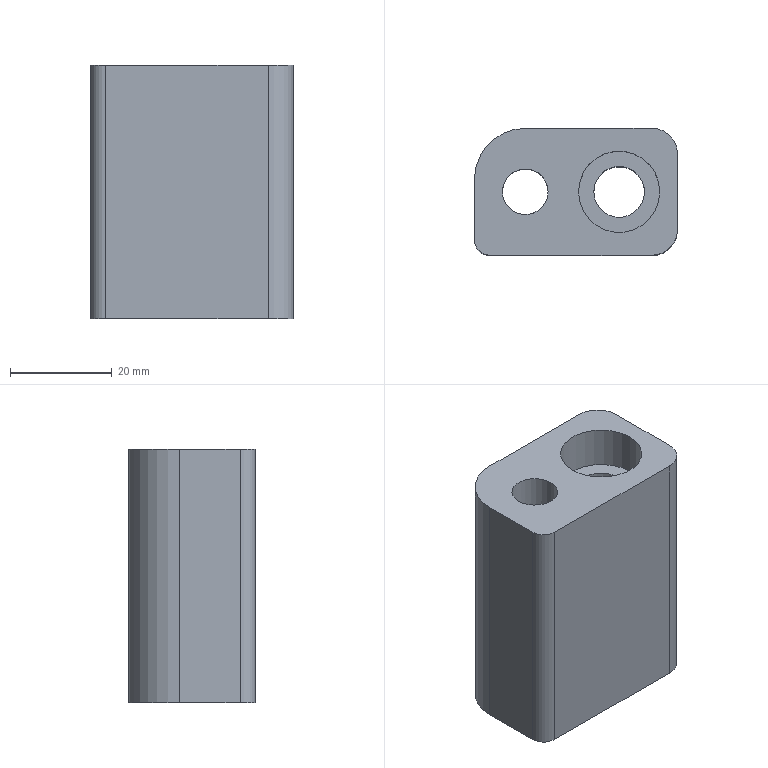Part | STEP file | PN_0016_id882_x_t | 1 solid | 16 faces | box 40 x 25 x 50 mm | volume 37460 mm3 | plane 8 | cylinder 8 | commonest cylinder face diameters 10 x3 6 x1 9 x1 14 x1 16 x1 20 x1
STEP:
#1=CARTESIAN_POINT('',(-201.,0.,95.));
#2=VERTEX_POINT('',#1);
#3=CARTESIAN_POINT('',(-209.,0.,95.));
#4=DIRECTION('',(0.,0.,-1.));
#5=DIRECTION('',(1.,0.,0.));
#6=AXIS2_PLACEMENT_3D('',#3,#4,#5);
#7=CIRCLE('',#6,8.);
#8=EDGE_CURVE('',#2,#2,#7,.T.);
#9=ORIENTED_EDGE('',*,*,#8,.T.);
#10=EDGE_LOOP('',(#9));
#11=FACE_BOUND('',#10,.T.);
#12=CARTESIAN_POINT('',(-223.,0.,95.));
#13=VERTEX_POINT('',#12);
#14=CARTESIAN_POINT('',(-227.5,0.,95.));
#15=DIRECTION('',(0.,0.,1.));
#16=DIRECTION('',(1.,0.,0.));
#17=AXIS2_PLACEMENT_3D('',#14,#15,#16);
#18=CIRCLE('',#17,4.5);
#19=EDGE_CURVE('',#13,#13,#18,.T.);
#20=ORIENTED_EDGE('',*,*,#19,.F.);
#21=EDGE_LOOP('',(#20));
#22=FACE_BOUND('',#21,.T.);
#23=CARTESIAN_POINT('',(-237.5,-9.5,95.));
#24=VERTEX_POINT('',#23);
#25=CARTESIAN_POINT('',(-237.5,2.5,95.));
#26=VERTEX_POINT('',#25);
#27=CARTESIAN_POINT('',(-237.5,0.,95.));
#28=DIRECTION('',(0.,1.,0.));
#29=VECTOR('',#28,1.);
#30=LINE('',#27,#29);
#31=EDGE_CURVE('',#24,#26,#30,.T.);
#32=ORIENTED_EDGE('',*,*,#31,.F.);
#33=CARTESIAN_POINT('',(-234.5,-12.5,95.));
#34=VERTEX_POINT('',#33);
#35=CARTESIAN_POINT('',(-234.5,-9.5,95.));
#36=DIRECTION('',(0.,0.,1.));
#37=DIRECTION('',(1.,0.,0.));
#38=AXIS2_PLACEMENT_3D('',#35,#36,#37);
#39=CIRCLE('',#38,3.);
#40=EDGE_CURVE('',#24,#34,#39,.T.);
#41=ORIENTED_EDGE('',*,*,#40,.T.);
#42=CARTESIAN_POINT('',(-202.5,-12.5,95.));
#43=VERTEX_POINT('',#42);
#44=CARTESIAN_POINT('',(-209.,-12.5,95.));
#45=DIRECTION('',(-1.,0.,0.));
#46=VECTOR('',#45,1.);
#47=LINE('',#44,#46);
#48=EDGE_CURVE('',#43,#34,#47,.T.);
#49=ORIENTED_EDGE('',*,*,#48,.F.);
#50=CARTESIAN_POINT('',(-197.5,-7.5,95.));
#51=VERTEX_POINT('',#50);
#52=CARTESIAN_POINT('',(-202.5,-7.5,95.));
#53=DIRECTION('',(0.,0.,1.));
#54=DIRECTION('',(1.,0.,0.));
#55=AXIS2_PLACEMENT_3D('',#52,#53,#54);
#56=CIRCLE('',#55,5.);
#57=EDGE_CURVE('',#43,#51,#56,.T.);
#58=ORIENTED_EDGE('',*,*,#57,.T.);
#59=CARTESIAN_POINT('',(-197.5,7.5,95.));
#60=VERTEX_POINT('',#59);
#61=CARTESIAN_POINT('',(-197.5,0.,95.));
#62=DIRECTION('',(0.,-1.,0.));
#63=VECTOR('',#62,1.);
#64=LINE('',#61,#63);
#65=EDGE_CURVE('',#60,#51,#64,.T.);
#66=ORIENTED_EDGE('',*,*,#65,.F.);
#67=CARTESIAN_POINT('',(-202.5,12.5,95.));
#68=VERTEX_POINT('',#67);
#69=CARTESIAN_POINT('',(-202.5,7.5,95.));
#70=DIRECTION('',(0.,0.,1.));
#71=DIRECTION('',(1.,0.,0.));
#72=AXIS2_PLACEMENT_3D('',#69,#70,#71);
#73=CIRCLE('',#72,5.);
#74=EDGE_CURVE('',#60,#68,#73,.T.);
#75=ORIENTED_EDGE('',*,*,#74,.T.);
#76=CARTESIAN_POINT('',(-227.5,12.5,95.));
#77=VERTEX_POINT('',#76);
#78=CARTESIAN_POINT('',(-209.,12.5,95.));
#79=DIRECTION('',(1.,0.,0.));
#80=VECTOR('',#79,1.);
#81=LINE('',#78,#80);
#82=EDGE_CURVE('',#77,#68,#81,.T.);
#83=ORIENTED_EDGE('',*,*,#82,.F.);
#84=CARTESIAN_POINT('',(-227.5,2.5,95.));
#85=DIRECTION('',(0.,0.,1.));
#86=DIRECTION('',(1.,0.,0.));
#87=AXIS2_PLACEMENT_3D('',#84,#85,#86);
#88=CIRCLE('',#87,10.);
#89=EDGE_CURVE('',#77,#26,#88,.T.);
#90=ORIENTED_EDGE('',*,*,#89,.T.);
#91=EDGE_LOOP('',(#32,#41,#49,#58,#66,#75,#83,#90));
#92=FACE_BOUND('',#91,.T.);
#93=CARTESIAN_POINT('',(-209.,0.,95.));
#94=DIRECTION('',(0.,0.,1.));
#95=DIRECTION('',(0.,-1.,0.));
#96=AXIS2_PLACEMENT_3D('',#93,#94,#95);
#97=PLANE('',#96);
#98=ADVANCED_FACE('',(#11,#22,#92),#97,.T.);
#99=CARTESIAN_POINT('',(-237.5,2.5,45.));
#100=VERTEX_POINT('',#99);
#101=CARTESIAN_POINT('',(-237.5,-9.5,45.));
#102=VERTEX_POINT('',#101);
#103=CARTESIAN_POINT('',(-237.5,0.,45.));
#104=DIRECTION('',(0.,-1.,0.));
#105=VECTOR('',#104,1.);
#106=LINE('',#103,#105);
#107=EDGE_CURVE('',#100,#102,#106,.T.);
#108=ORIENTED_EDGE('',*,*,#107,.T.);
#109=CARTESIAN_POINT('',(-237.5,-9.5,5.));
#110=DIRECTION('',(0.,0.,1.));
#111=VECTOR('',#110,1.);
#112=LINE('',#109,#111);
#113=EDGE_CURVE('',#102,#24,#112,.T.);
#114=ORIENTED_EDGE('',*,*,#113,.T.);
#115=ORIENTED_EDGE('',*,*,#31,.T.);
#116=CARTESIAN_POINT('',(-237.5,2.5,5.));
#117=DIRECTION('',(0.,0.,-1.));
#118=VECTOR('',#117,1.);
#119=LINE('',#116,#118);
#120=EDGE_CURVE('',#26,#100,#119,.T.);
#121=ORIENTED_EDGE('',*,*,#120,.T.);
#122=EDGE_LOOP('',(#108,#114,#115,#121));
#123=FACE_OUTER_BOUND('',#122,.T.);
#124=CARTESIAN_POINT('',(-237.5,0.,5.));
#125=DIRECTION('',(-1.,0.,0.));
#126=DIRECTION('',(0.,0.,-1.));
#127=AXIS2_PLACEMENT_3D('',#124,#125,#126);
#128=PLANE('',#127);
#129=ADVANCED_FACE('',(#123),#128,.T.);
#130=CARTESIAN_POINT('',(-202.5,12.5,45.));
#131=VERTEX_POINT('',#130);
#132=CARTESIAN_POINT('',(-227.5,12.5,45.));
#133=VERTEX_POINT('',#132);
#134=CARTESIAN_POINT('',(-209.,12.5,45.));
#135=DIRECTION('',(-1.,0.,0.));
#136=VECTOR('',#135,1.);
#137=LINE('',#134,#136);
#138=EDGE_CURVE('',#131,#133,#137,.T.);
#139=ORIENTED_EDGE('',*,*,#138,.T.);
#140=CARTESIAN_POINT('',(-227.5,12.5,5.));
#141=DIRECTION('',(0.,0.,1.));
#142=VECTOR('',#141,1.);
#143=LINE('',#140,#142);
#144=EDGE_CURVE('',#133,#77,#143,.T.);
#145=ORIENTED_EDGE('',*,*,#144,.T.);
#146=ORIENTED_EDGE('',*,*,#82,.T.);
#147=CARTESIAN_POINT('',(-202.5,12.5,5.));
#148=DIRECTION('',(0.,0.,-1.));
#149=VECTOR('',#148,1.);
#150=LINE('',#147,#149);
#151=EDGE_CURVE('',#68,#131,#150,.T.);
#152=ORIENTED_EDGE('',*,*,#151,.T.);
#153=EDGE_LOOP('',(#139,#145,#146,#152));
#154=FACE_OUTER_BOUND('',#153,.T.);
#155=CARTESIAN_POINT('',(-209.,12.5,5.));
#156=DIRECTION('',(0.,1.,0.));
#157=DIRECTION('',(0.,0.,1.));
#158=AXIS2_PLACEMENT_3D('',#155,#156,#157);
#159=PLANE('',#158);
#160=ADVANCED_FACE('',(#154),#159,.T.);
#161=ORIENTED_EDGE('',*,*,#65,.T.);
#162=CARTESIAN_POINT('',(-197.5,-7.5,45.));
#163=VERTEX_POINT('',#162);
#164=CARTESIAN_POINT('',(-197.5,-7.5,5.));
#165=DIRECTION('',(0.,0.,-1.));
#166=VECTOR('',#165,1.);
#167=LINE('',#164,#166);
#168=EDGE_CURVE('',#51,#163,#167,.T.);
#169=ORIENTED_EDGE('',*,*,#168,.T.);
#170=CARTESIAN_POINT('',(-197.5,7.5,45.));
#171=VERTEX_POINT('',#170);
#172=CARTESIAN_POINT('',(-197.5,0.,45.));
#173=DIRECTION('',(0.,1.,0.));
#174=VECTOR('',#173,1.);
#175=LINE('',#172,#174);
#176=EDGE_CURVE('',#163,#171,#175,.T.);
#177=ORIENTED_EDGE('',*,*,#176,.T.);
#178=CARTESIAN_POINT('',(-197.5,7.5,5.));
#179=DIRECTION('',(0.,0.,1.));
#180=VECTOR('',#179,1.);
#181=LINE('',#178,#180);
#182=EDGE_CURVE('',#171,#60,#181,.T.);
#183=ORIENTED_EDGE('',*,*,#182,.T.);
#184=EDGE_LOOP('',(#161,#169,#177,#183));
#185=FACE_OUTER_BOUND('',#184,.T.);
#186=CARTESIAN_POINT('',(-197.5,0.,5.));
#187=DIRECTION('',(1.,0.,0.));
#188=DIRECTION('',(0.,0.,1.));
#189=AXIS2_PLACEMENT_3D('',#186,#187,#188);
#190=PLANE('',#189);
#191=ADVANCED_FACE('',(#185),#190,.T.);
#192=CARTESIAN_POINT('',(-204.,0.,45.));
#193=VERTEX_POINT('',#192);
#194=CARTESIAN_POINT('',(-209.,0.,45.));
#195=DIRECTION('',(0.,0.,1.));
#196=DIRECTION('',(1.,0.,0.));
#197=AXIS2_PLACEMENT_3D('',#194,#195,#196);
#198=CIRCLE('',#197,5.);
#199=EDGE_CURVE('',#193,#193,#198,.T.);
#200=ORIENTED_EDGE('',*,*,#199,.T.);
#201=EDGE_LOOP('',(#200));
#202=FACE_BOUND('',#201,.T.);
#203=CARTESIAN_POINT('',(-227.5,-7.,45.));
#204=VERTEX_POINT('',#203);
#205=CARTESIAN_POINT('',(-227.5,0.,45.));
#206=DIRECTION('',(0.,0.,1.));
#207=DIRECTION('',(0.,-1.,0.));
#208=AXIS2_PLACEMENT_3D('',#205,#206,#207);
#209=CIRCLE('',#208,7.);
#210=EDGE_CURVE('',#204,#204,#209,.T.);
#211=ORIENTED_EDGE('',*,*,#210,.T.);
#212=EDGE_LOOP('',(#211));
#213=FACE_BOUND('',#212,.T.);
#214=CARTESIAN_POINT('',(-234.5,-12.5,45.));
#215=VERTEX_POINT('',#214);
#216=CARTESIAN_POINT('',(-202.5,-12.5,45.));
#217=VERTEX_POINT('',#216);
#218=CARTESIAN_POINT('',(-209.,-12.5,45.));
#219=DIRECTION('',(1.,0.,0.));
#220=VECTOR('',#219,1.);
#221=LINE('',#218,#220);
#222=EDGE_CURVE('',#215,#217,#221,.T.);
#223=ORIENTED_EDGE('',*,*,#222,.F.);
#224=CARTESIAN_POINT('',(-234.5,-9.5,45.));
#225=DIRECTION('',(0.,0.,-1.));
#226=DIRECTION('',(1.,0.,0.));
#227=AXIS2_PLACEMENT_3D('',#224,#225,#226);
#228=CIRCLE('',#227,3.);
#229=EDGE_CURVE('',#215,#102,#228,.T.);
#230=ORIENTED_EDGE('',*,*,#229,.T.);
#231=ORIENTED_EDGE('',*,*,#107,.F.);
#232=CARTESIAN_POINT('',(-227.5,2.5,45.));
#233=DIRECTION('',(0.,0.,-1.));
#234=DIRECTION('',(1.,0.,0.));
#235=AXIS2_PLACEMENT_3D('',#232,#233,#234);
#236=CIRCLE('',#235,10.);
#237=EDGE_CURVE('',#100,#133,#236,.T.);
#238=ORIENTED_EDGE('',*,*,#237,.T.);
#239=ORIENTED_EDGE('',*,*,#138,.F.);
#240=CARTESIAN_POINT('',(-202.5,7.5,45.));
#241=DIRECTION('',(0.,0.,-1.));
#242=DIRECTION('',(1.,0.,0.));
#243=AXIS2_PLACEMENT_3D('',#240,#241,#242);
#244=CIRCLE('',#243,5.);
#245=EDGE_CURVE('',#131,#171,#244,.T.);
#246=ORIENTED_EDGE('',*,*,#245,.T.);
#247=ORIENTED_EDGE('',*,*,#176,.F.);
#248=CARTESIAN_POINT('',(-202.5,-7.5,45.));
#249=DIRECTION('',(0.,0.,-1.));
#250=DIRECTION('',(1.,0.,0.));
#251=AXIS2_PLACEMENT_3D('',#248,#249,#250);
#252=CIRCLE('',#251,5.);
#253=EDGE_CURVE('',#163,#217,#252,.T.);
#254=ORIENTED_EDGE('',*,*,#253,.T.);
#255=EDGE_LOOP('',(#223,#230,#231,#238,#239,#246,#247,#254));
#256=FACE_BOUND('',#255,.T.);
#257=CARTESIAN_POINT('',(-192.,-125.189,45.));
#258=DIRECTION('',(0.,0.,1.));
#259=DIRECTION('',(0.,-1.,0.));
#260=AXIS2_PLACEMENT_3D('',#257,#258,#259);
#261=PLANE('',#260);
#262=ADVANCED_FACE('',(#202,#213,#256),#261,.F.);
#263=ORIENTED_EDGE('',*,*,#48,.T.);
#264=CARTESIAN_POINT('',(-234.5,-12.5,5.));
#265=DIRECTION('',(0.,0.,-1.));
#266=VECTOR('',#265,1.);
#267=LINE('',#264,#266);
#268=EDGE_CURVE('',#34,#215,#267,.T.);
#269=ORIENTED_EDGE('',*,*,#268,.T.);
#270=ORIENTED_EDGE('',*,*,#222,.T.);
#271=CARTESIAN_POINT('',(-202.5,-12.5,5.));
#272=DIRECTION('',(0.,0.,1.));
#273=VECTOR('',#272,1.);
#274=LINE('',#271,#273);
#275=EDGE_CURVE('',#217,#43,#274,.T.);
#276=ORIENTED_EDGE('',*,*,#275,.T.);
#277=EDGE_LOOP('',(#263,#269,#270,#276));
#278=FACE_OUTER_BOUND('',#277,.T.);
#279=CARTESIAN_POINT('',(-209.,-12.5,5.));
#280=DIRECTION('',(0.,-1.,0.));
#281=DIRECTION('',(0.,0.,-1.));
#282=AXIS2_PLACEMENT_3D('',#279,#280,#281);
#283=PLANE('',#282);
#284=ADVANCED_FACE('',(#278),#283,.T.);
#285=ORIENTED_EDGE('',*,*,#253,.F.);
#286=ORIENTED_EDGE('',*,*,#168,.F.);
#287=ORIENTED_EDGE('',*,*,#57,.F.);
#288=ORIENTED_EDGE('',*,*,#275,.F.);
#289=EDGE_LOOP('',(#285,#286,#287,#288));
#290=FACE_OUTER_BOUND('',#289,.T.);
#291=CARTESIAN_POINT('',(-202.5,-7.5,5.));
#292=DIRECTION('',(0.,0.,1.));
#293=DIRECTION('',(1.,0.,0.));
#294=AXIS2_PLACEMENT_3D('',#291,#292,#293);
#295=CYLINDRICAL_SURFACE('',#294,5.);
#296=ADVANCED_FACE('',(#290),#295,.T.);
#297=ORIENTED_EDGE('',*,*,#245,.F.);
#298=ORIENTED_EDGE('',*,*,#151,.F.);
#299=ORIENTED_EDGE('',*,*,#74,.F.);
#300=ORIENTED_EDGE('',*,*,#182,.F.);
#301=EDGE_LOOP('',(#297,#298,#299,#300));
#302=FACE_OUTER_BOUND('',#301,.T.);
#303=CARTESIAN_POINT('',(-202.5,7.5,5.));
#304=DIRECTION('',(0.,0.,1.));
#305=DIRECTION('',(1.,0.,0.));
#306=AXIS2_PLACEMENT_3D('',#303,#304,#305);
#307=CYLINDRICAL_SURFACE('',#306,5.);
#308=ADVANCED_FACE('',(#302),#307,.T.);
#309=ORIENTED_EDGE('',*,*,#237,.F.);
#310=ORIENTED_EDGE('',*,*,#120,.F.);
#311=ORIENTED_EDGE('',*,*,#89,.F.);
#312=ORIENTED_EDGE('',*,*,#144,.F.);
#313=EDGE_LOOP('',(#309,#310,#311,#312));
#314=FACE_OUTER_BOUND('',#313,.T.);
#315=CARTESIAN_POINT('',(-227.5,2.5,5.));
#316=DIRECTION('',(0.,0.,1.));
#317=DIRECTION('',(1.,0.,0.));
#318=AXIS2_PLACEMENT_3D('',#315,#316,#317);
#319=CYLINDRICAL_SURFACE('',#318,10.);
#320=ADVANCED_FACE('',(#314),#319,.T.);
#321=ORIENTED_EDGE('',*,*,#229,.F.);
#322=ORIENTED_EDGE('',*,*,#268,.F.);
#323=ORIENTED_EDGE('',*,*,#40,.F.);
#324=ORIENTED_EDGE('',*,*,#113,.F.);
#325=EDGE_LOOP('',(#321,#322,#323,#324));
#326=FACE_OUTER_BOUND('',#325,.T.);
#327=CARTESIAN_POINT('',(-234.5,-9.5,5.));
#328=DIRECTION('',(0.,0.,1.));
#329=DIRECTION('',(1.,0.,0.));
#330=AXIS2_PLACEMENT_3D('',#327,#328,#329);
#331=CYLINDRICAL_SURFACE('',#330,3.);
#332=ADVANCED_FACE('',(#326),#331,.T.);
#333=ORIENTED_EDGE('',*,*,#19,.T.);
#334=EDGE_LOOP('',(#333));
#335=FACE_BOUND('',#334,.T.);
#336=CARTESIAN_POINT('',(-227.5,-4.5,75.));
#337=VERTEX_POINT('',#336);
#338=CARTESIAN_POINT('',(-227.5,0.,75.));
#339=DIRECTION('',(0.,0.,1.));
#340=DIRECTION('',(0.,-1.,0.));
#341=AXIS2_PLACEMENT_3D('',#338,#339,#340);
#342=CIRCLE('',#341,4.5);
#343=EDGE_CURVE('',#337,#337,#342,.T.);
#344=ORIENTED_EDGE('',*,*,#343,.F.);
#345=EDGE_LOOP('',(#344));
#346=FACE_BOUND('',#345,.T.);
#347=CARTESIAN_POINT('',(-227.5,0.,105.));
#348=DIRECTION('',(0.,0.,-1.));
#349=DIRECTION('',(0.,1.,0.));
#350=AXIS2_PLACEMENT_3D('',#347,#348,#349);
#351=CYLINDRICAL_SURFACE('',#350,4.5);
#352=ADVANCED_FACE('',(#335,#346),#351,.F.);
#353=ORIENTED_EDGE('',*,*,#343,.T.);
#354=EDGE_LOOP('',(#353));
#355=FACE_BOUND('',#354,.T.);
#356=CARTESIAN_POINT('',(-227.5,7.,75.));
#357=VERTEX_POINT('',#356);
#358=CARTESIAN_POINT('',(-227.5,0.,75.));
#359=DIRECTION('',(0.,0.,1.));
#360=DIRECTION('',(0.,1.,0.));
#361=AXIS2_PLACEMENT_3D('',#358,#359,#360);
#362=CIRCLE('',#361,7.);
#363=EDGE_CURVE('',#357,#357,#362,.T.);
#364=ORIENTED_EDGE('',*,*,#363,.F.);
#365=EDGE_LOOP('',(#364));
#366=FACE_BOUND('',#365,.T.);
#367=CARTESIAN_POINT('',(-227.5,0.,75.));
#368=DIRECTION('',(0.,0.,1.));
#369=DIRECTION('',(0.,-1.,0.));
#370=AXIS2_PLACEMENT_3D('',#367,#368,#369);
#371=PLANE('',#370);
#372=ADVANCED_FACE('',(#355,#366),#371,.F.);
#373=ORIENTED_EDGE('',*,*,#210,.F.);
#374=EDGE_LOOP('',(#373));
#375=FACE_BOUND('',#374,.T.);
#376=ORIENTED_EDGE('',*,*,#363,.T.);
#377=EDGE_LOOP('',(#376));
#378=FACE_BOUND('',#377,.T.);
#379=CARTESIAN_POINT('',(-227.5,0.,75.));
#380=DIRECTION('',(0.,0.,-1.));
#381=DIRECTION('',(0.,1.,0.));
#382=AXIS2_PLACEMENT_3D('',#379,#380,#381);
#383=CYLINDRICAL_SURFACE('',#382,7.);
#384=ADVANCED_FACE('',(#375,#378),#383,.F.);
#385=CARTESIAN_POINT('',(-214.,0.,86.7));
#386=VERTEX_POINT('',#385);
#387=CARTESIAN_POINT('',(-209.,0.,86.7));
#388=DIRECTION('',(0.,0.,-1.));
#389=DIRECTION('',(-1.,0.,0.));
#390=AXIS2_PLACEMENT_3D('',#387,#388,#389);
#391=CIRCLE('',#390,5.);
#392=EDGE_CURVE('',#386,#386,#391,.T.);
#393=ORIENTED_EDGE('',*,*,#392,.F.);
#394=EDGE_LOOP('',(#393));
#395=FACE_BOUND('',#394,.T.);
#396=ORIENTED_EDGE('',*,*,#199,.F.);
#397=EDGE_LOOP('',(#396));
#398=FACE_BOUND('',#397,.T.);
#399=CARTESIAN_POINT('',(-209.,0.,85.5));
#400=DIRECTION('',(0.,0.,-1.));
#401=DIRECTION('',(0.,-1.,0.));
#402=AXIS2_PLACEMENT_3D('',#399,#400,#401);
#403=CYLINDRICAL_SURFACE('',#402,5.);
#404=ADVANCED_FACE('',(#395,#398),#403,.F.);
#405=ORIENTED_EDGE('',*,*,#392,.T.);
#406=EDGE_LOOP('',(#405));
#407=FACE_BOUND('',#406,.T.);
#408=CARTESIAN_POINT('',(-217.,0.,86.7));
#409=VERTEX_POINT('',#408);
#410=CARTESIAN_POINT('',(-209.,0.,86.7));
#411=DIRECTION('',(0.,0.,-1.));
#412=DIRECTION('',(-1.,0.,0.));
#413=AXIS2_PLACEMENT_3D('',#410,#411,#412);
#414=CIRCLE('',#413,8.);
#415=EDGE_CURVE('',#409,#409,#414,.T.);
#416=ORIENTED_EDGE('',*,*,#415,.F.);
#417=EDGE_LOOP('',(#416));
#418=FACE_BOUND('',#417,.T.);
#419=CARTESIAN_POINT('',(-209.,0.,86.7));
#420=DIRECTION('',(0.,0.,-1.));
#421=DIRECTION('',(-1.,0.,0.));
#422=AXIS2_PLACEMENT_3D('',#419,#420,#421);
#423=PLANE('',#422);
#424=ADVANCED_FACE('',(#407,#418),#423,.F.);
#425=ORIENTED_EDGE('',*,*,#415,.T.);
#426=EDGE_LOOP('',(#425));
#427=FACE_BOUND('',#426,.T.);
#428=ORIENTED_EDGE('',*,*,#8,.F.);
#429=EDGE_LOOP('',(#428));
#430=FACE_BOUND('',#429,.T.);
#431=CARTESIAN_POINT('',(-209.,0.,94.559));
#432=DIRECTION('',(0.,0.,-1.));
#433=DIRECTION('',(0.,-1.,0.));
#434=AXIS2_PLACEMENT_3D('',#431,#432,#433);
#435=CYLINDRICAL_SURFACE('',#434,8.);
#436=ADVANCED_FACE('',(#427,#430),#435,.F.);
#437=CLOSED_SHELL('',(#98,#129,#160,#191,#262,#284,#296,#308,#320,#332,#352,#372,#384,#404,#424,#436));
#438=MANIFOLD_SOLID_BREP('',#437);
#439=(LENGTH_UNIT()NAMED_UNIT(*)SI_UNIT(.MILLI.,.METRE.));
#440=UNCERTAINTY_MEASURE_WITH_UNIT(LENGTH_MEASURE(0.00002),#439,'','');
#441=(NAMED_UNIT(*)PLANE_ANGLE_UNIT()SI_UNIT($,.RADIAN.));
#442=PLANE_ANGLE_MEASURE_WITH_UNIT(PLANE_ANGLE_MEASURE(0.01745),#441);
#443=DIMENSIONAL_EXPONENTS(0.,0.,0.,0.,0.,0.,0.);
#444=(CONVERSION_BASED_UNIT('DEGREE',#442)NAMED_UNIT(#443)PLANE_ANGLE_UNIT());
#445=(NAMED_UNIT(*)SI_UNIT($,.STERADIAN.)SOLID_ANGLE_UNIT());
#446=(GEOMETRIC_REPRESENTATION_CONTEXT(3)GLOBAL_UNCERTAINTY_ASSIGNED_CONTEXT((#440))GLOBAL_UNIT_ASSIGNED_CONTEXT((#439,#444,#445))REPRESENTATION_CONTEXT('',''));
#447=ADVANCED_BREP_SHAPE_REPRESENTATION('',(#438),#446);